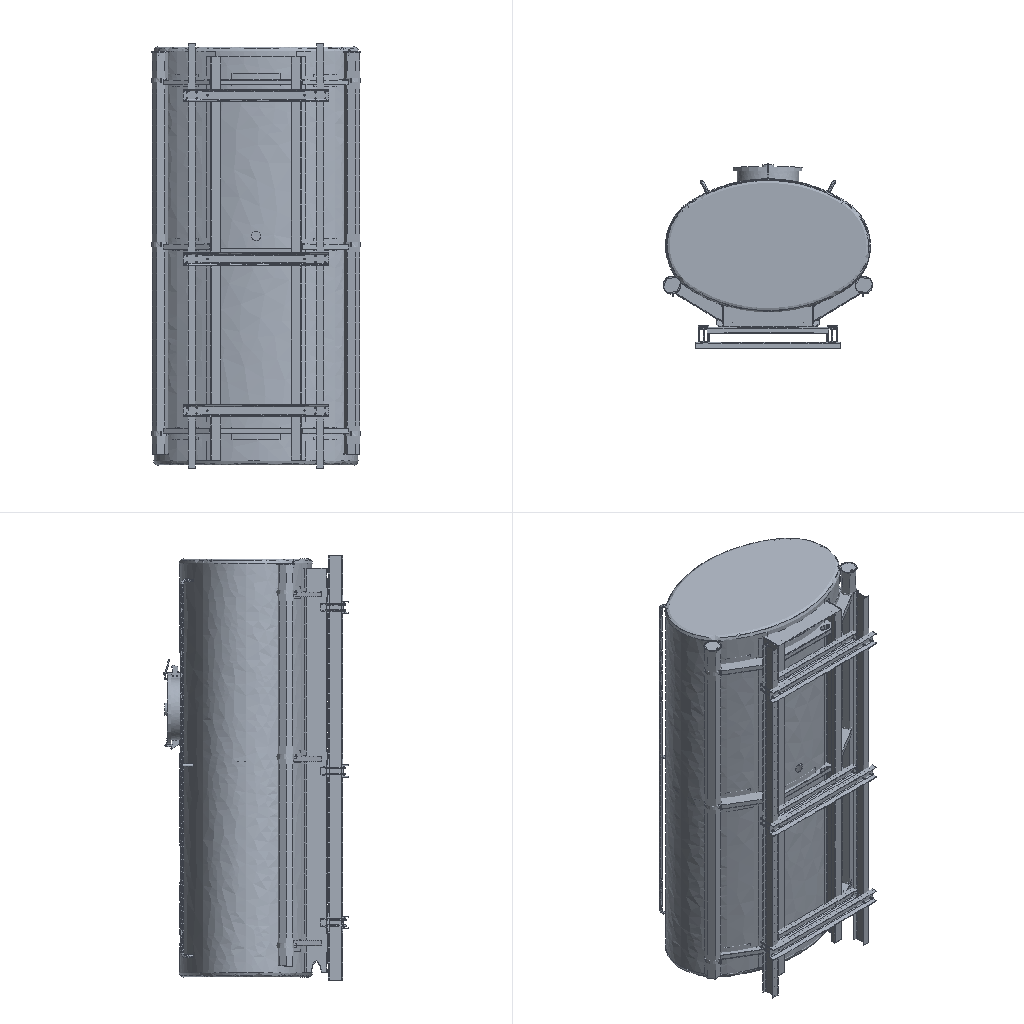Simulation study | ansys workbench
Ansys APDL input file, long lists of numbers shortened:
/batch
/config,noeldb,1     ! force off writing results to database
*get,_wallstrt,active,,time,wall
! ANSYS input file written by Workbench version 2022 R1
! File used for geometry attach: F:\ansys（分析文件汇总)\洒水车有限元分析\晒水车罐体.STEP
/title,wbnew--____ 2 (E5)
! ****** Begin Custom Load Command Snippet ******
/COM, ACT Extensions:
/COM,     LSDYNA, 2021.1
/COM,
! ****** End   Custom Load Command Snippet ******
*DIM,_wb_ProjectScratch_dir,string,248
_wb_ProjectScratch_dir(1) = 'C:\Users\Administrator\AppData\Local\Temp\WB_Administrator_19044_2\_ProjectScratch\Scr5F41\'
*DIM,_wb_SolverFiles_dir,string,248
_wb_SolverFiles_dir(1) = 'C:\Users\Administrator\AppData\Local\Temp\WB_Administrator_19044_2\wbnew_files\dp0\SYS-3\MECH\'
*DIM,_wb_userfiles_dir,string,248
_wb_userfiles_dir(1) = 'C:\Users\Administrator\AppData\Local\Temp\WB_Administrator_19044_2\wbnew_files\user_files\'
/com,--- Data in consistent NMM units. See Solving Units in the help system for more information.
/units,MPA
/nopr
/wb,file,start              !  signify a WB generated input file
/prep7
! Turn off shape checking because checks already performed inside WB mesher.
! See help system for more information.
SHPP,OFF,,NOWARN
/nolist
etcon,set             ! allow ANSYS to choose best KEYOP's for 180x elements, resets any applicable keyopt to MAPDL defaults
/com,*********** Nodes for the whole assembly ***********
nblock,3,,154514
(1i9,3e20.9e3)
    59613    -4.978285790E+02     4.306437121E+02     3.184288870E+01
! (140467 more lines like these left out)
-1
/wb,elem,start            !  set before creation of elements
/com,*********** Elements for Body 1 "__|1210-011-G03|__-__1" ***********
et,1,187
eblock,19,solid,,5134
(19i9)
        1        1        1        1        0        0        0        0       10        0        1     1367     1730     1457     1374     9329     9682     9325     9324
! (10267 more lines like these left out)
-1
/com,*********** Elements for Body 2 "__|1210-011-G03|__-__1[2]" ***********
et,2,187
eblock,19,solid,,5134
(19i9)
        2        2        2        2        0        0        0        0       10        0     5135    12093    12456    12183    12100    20055    20408    20051    20050
! (10267 more lines like these left out)
-1
/com,*********** Elements for Body 3 "__|__-0|__-__3" ***********
et,3,187
eblock,19,solid,,12299
(19i9)
        3        3        3        3        0        0        0        0       10        0    10269    22599    23787    23678    22852    33647    40850    33645    33640
! (24597 more lines like these left out)
-1
/com,*********** Elements for Body 4 "__|1210-041-G03|__-__9" ***********
et,4,187
eblock,19,solid,,1630
(19i9)
        4        4        4        4        0        0        0        0       10        0    22568    46545    47052    46995    46688    47336    49436    47333    47330
! (3259 more lines like these left out)
-1
/com,*********** Elements for Body 5 "__|1210-042-G03|__-__1" ***********
et,5,186
keyo,5,2,1          ! set full integration on SOLID186
eblock,19,solid,,62
(19i9)
        5        5        5        5        0        0        0        0       20        0    24198    50489    50500    50499    50490    50548    50537    50538    50539
! (123 more lines like these left out)
-1
! (74 more sections like these left out)
/wb,elem,end               !  done creating elements
/com,*********** Send User Defined Coordinate System(s) ***********
csys,0
toffst,273.15,  ! Temperature offset from absolute zero
/com,*********** Set Reference Temperature ***********
tref,22.
/wb,mat,start              !  starting to send materials
/com,*********** Send Materials ***********
Temperature = 'TEMP' ! Temperature
MP,DENS,1,7.85e-09,	! tonne mm^-3
MP,ALPX,1,1.2e-05,	! C^-1
MP,C,1,434000000,	! mm^2 s^-2 C^-1
MP,KXX,1,60.5,	! tonne mm s^-3 C^-1
MP,RSVX,1,0.00017,	! ohm mm
MP,EX,1,200000,	! tonne s^-2 mm^-1
MP,NUXY,1,0.3,
MP,MURX,1,10000,
Temperature = 'TEMP' ! Temperature
MP,DENS,2,7.85e-09,	! tonne mm^-3
MP,ALPX,2,1.2e-05,	! C^-1
MP,C,2,434000000,	! mm^2 s^-2 C^-1
MP,KXX,2,60.5,	! tonne mm s^-3 C^-1
MP,RSVX,2,0.00017,	! ohm mm
MP,EX,2,200000,	! tonne s^-2 mm^-1
MP,NUXY,2,0.3,
MP,MURX,2,10000,
Temperature = 'TEMP' ! Temperature
MP,DENS,3,7.85e-09,	! tonne mm^-3
MP,ALPX,3,1.2e-05,	! C^-1
MP,C,3,434000000,	! mm^2 s^-2 C^-1
MP,KXX,3,60.5,	! tonne mm s^-3 C^-1
MP,RSVX,3,0.00017,	! ohm mm
MP,EX,3,200000,	! tonne s^-2 mm^-1
MP,NUXY,3,0.3,
MP,MURX,3,10000,
Temperature = 'TEMP' ! Temperature
MP,DENS,4,7.85e-09,	! tonne mm^-3
MP,ALPX,4,1.2e-05,	! C^-1
MP,C,4,434000000,	! mm^2 s^-2 C^-1
MP,KXX,4,60.5,	! tonne mm s^-3 C^-1
MP,RSVX,4,0.00017,	! ohm mm
MP,EX,4,200000,	! tonne s^-2 mm^-1
MP,NUXY,4,0.3,
MP,MURX,4,10000,
Temperature = 'TEMP' ! Temperature
MP,DENS,5,7.85e-09,	! tonne mm^-3
MP,ALPX,5,1.2e-05,	! C^-1
MP,C,5,434000000,	! mm^2 s^-2 C^-1
MP,KXX,5,60.5,	! tonne mm s^-3 C^-1
MP,RSVX,5,0.00017,	! ohm mm
MP,EX,5,200000,	! tonne s^-2 mm^-1
MP,NUXY,5,0.3,
MP,MURX,5,10000,
Temperature = 'TEMP' ! Temperature
MP,DENS,6,7.85e-09,	! tonne mm^-3
MP,ALPX,6,1.2e-05,	! C^-1
MP,C,6,434000000,	! mm^2 s^-2 C^-1
MP,KXX,6,60.5,	! tonne mm s^-3 C^-1
MP,RSVX,6,0.00017,	! ohm mm
MP,EX,6,200000,	! tonne s^-2 mm^-1
MP,NUXY,6,0.3,
MP,MURX,6,10000,
Temperature = 'TEMP' ! Temperature
MP,DENS,7,7.85e-09,	! tonne mm^-3
MP,ALPX,7,1.2e-05,	! C^-1
MP,C,7,434000000,	! mm^2 s^-2 C^-1
MP,KXX,7,60.5,	! tonne mm s^-3 C^-1
MP,RSVX,7,0.00017,	! ohm mm
MP,EX,7,200000,	! tonne s^-2 mm^-1
MP,NUXY,7,0.3,
MP,MURX,7,10000,
Temperature = 'TEMP' ! Temperature
MP,DENS,8,7.85e-09,	! tonne mm^-3
MP,ALPX,8,1.2e-05,	! C^-1
MP,C,8,434000000,	! mm^2 s^-2 C^-1
MP,KXX,8,60.5,	! tonne mm s^-3 C^-1
MP,RSVX,8,0.00017,	! ohm mm
MP,EX,8,200000,	! tonne s^-2 mm^-1
MP,NUXY,8,0.3,
MP,MURX,8,10000,
Temperature = 'TEMP' ! Temperature
MP,DENS,9,7.85e-09,	! tonne mm^-3
MP,ALPX,9,1.2e-05,	! C^-1
MP,C,9,434000000,	! mm^2 s^-2 C^-1
MP,KXX,9,60.5,	! tonne mm s^-3 C^-1
MP,RSVX,9,0.00017,	! ohm mm
MP,EX,9,200000,	! tonne s^-2 mm^-1
! (632 more lines like these left out)
/wb,mat,end                !  done sending materials
!************************* Model Summary ********************
!__|1210-011-G03|__-__1,	Q235B,	matid,	1
!__|1210-011-G03|__-__1[2],	Q235B,	matid,	2
!__|__-0|__-__3,	Q235B,	matid,	3
! (78 more lines like these left out)
*get,_xmin,node,,mnloc,x
*get,_ymin,node,,mnloc,y
*get,_zmin,node,,mnloc,z
*get,_xmax,node,,mxloc,x
*get,_ymax,node,,mxloc,y
*get,_zmax,node,,mxloc,z
_ASMDIAG=(_xmax-_xmin)*(_xmax-_xmin)+(_ymax-_ymin)*(_ymax-_ymin)+(_zmax-_zmin)*(_zmax-_zmin)
_ASMDIAG=SQRT(_ASMDIAG)
/wb,contact,start          !  starting to send contact
/com,*********** Create Contact "接触区域" ***********
/com,            Real Constant Set For Above Contact Is 81 & 80
*set,tid,81
*set,cid,80
r,tid
r,cid
et,tid,170
et,cid,174
eblock,10,,,316
(15i9)
   106793       81       81       81        0      240      526      550      550     3708     5545      550     3709
! (315 more lines like these left out)
-1
eblock,10,,,316
(15i9)
   107109       80       80       80        0      240      526      550      550     3708     5545      550     3709
! (315 more lines like these left out)
-1
eblock,10,,,119
(15i9)
   107425       80       81       80        0    21474    21805    21997    21997    25860    28558    21997    25861
! (118 more lines like these left out)
-1
eblock,10,,,119
(15i9)
   107544       81       80       81        0    21474    21805    21997    21997    25860    28558    21997    25861
! (118 more lines like these left out)
-1
keyo,cid,8,2               ! auto create asymmetric contact (from Program Controlled setting)
keyo,cid,10,0              ! adjust contact stiffness each NR iteration (from Program Controlled setting)
keyo,cid,12,5              ! bonded always
keyo,cid,18,1              ! small sliding turned on by application
keyo,cid,2,0               ! augmented Lagrange (from Program Controlled setting)
keyo,cid,4,0               ! on Gauss point (from Program Controlled setting)
keyo,cid,9,1               ! ignore initial gaps/penetration
keyo,cid,7,0               ! No Prediction
rmod,tid,3,10.      ! FKN
rmod,tid,5,0.       ! ICONT
rmod,tid,6,0.       ! PINB
rmod,tid,10,0.      ! CNOF
rmod,tid,12,0.      ! FKT
rmod,tid,36,260     ! WB DSID
rmod,cid,3,10.      ! FKN
rmod,cid,5,0.       ! ICONT
rmod,cid,6,0.       ! PINB
rmod,cid,10,0.      ! CNOF
rmod,cid,12,0.      ! FKT
rmod,cid,36,260     ! WB DSID
/com,*********** Create Contact "接触区域 2" ***********
/com,            Real Constant Set For Above Contact Is 83 & 82
*set,tid,83
*set,cid,82
r,tid
r,cid
et,tid,170
et,cid,174
eblock,10,,,10
(15i9)
   107663       83       83       83        0      221      499      516      516     3552     5438      516     3554
! (9 more lines like these left out)
-1
eblock,10,,,10
(15i9)
   107673       82       82       82        0      221      499      516      516     3552     5438      516     3554
! (9 more lines like these left out)
-1
eblock,10,,,2
(15i9)
   107683       82       83       82        0    63922    63923    63749    63747    64830    64280    64275    64276
   107684       82       83       82        0    63923    64008    63748    63749    64835    64279    64277    64280
-1
eblock,10,,,2
(15i9)
   107685       83       82       83        0    63922    63923    63749    63747    64830    64280    64275    64276
   107686       83       82       83        0    63923    64008    63748    63749    64835    64279    64277    64280
-1
keyo,cid,8,2               ! auto create asymmetric contact (from Program Controlled setting)
keyo,cid,10,0              ! adjust contact stiffness each NR iteration (from Program Controlled setting)
keyo,cid,12,5              ! bonded always
keyo,cid,18,1              ! small sliding turned on by application
keyo,cid,2,0               ! augmented Lagrange (from Program Controlled setting)
keyo,cid,4,0               ! on Gauss point (from Program Controlled setting)
keyo,cid,9,1               ! ignore initial gaps/penetration
keyo,cid,7,0               ! No Prediction
rmod,tid,3,10.      ! FKN
rmod,tid,5,0.       ! ICONT
rmod,tid,6,0.       ! PINB
rmod,tid,10,0.      ! CNOF
rmod,tid,12,0.      ! FKT
rmod,tid,36,263     ! WB DSID
rmod,cid,3,10.      ! FKN
rmod,cid,5,0.       ! ICONT
rmod,cid,6,0.       ! PINB
rmod,cid,10,0.      ! CNOF
rmod,cid,12,0.      ! FKT
rmod,cid,36,263     ! WB DSID
/com,*********** Create Contact "接触区域 3" ***********
/com,            Real Constant Set For Above Contact Is 85 & 84
*set,tid,85
*set,cid,84
r,tid
r,cid
et,tid,170
et,cid,174
eblock,10,,,27
(15i9)
   107687       85       85       85        0      221      499      516      516     3552     5438      516     3554
! (26 more lines like these left out)
-1
eblock,10,,,27
(15i9)
   107714       84       84       84        0      221      499      516      516     3552     5438      516     3554
! (26 more lines like these left out)
-1
eblock,10,,,173
(15i9)
   107741       84       85       84        0    65546    65628    65630    65630    65873    66412    65630    65874
! (172 more lines like these left out)
-1
eblock,10,,,173
(15i9)
   107914       85       84       85        0    65546    65628    65630    65630    65873    66412    65630    65874
! (172 more lines like these left out)
-1
keyo,cid,8,2               ! auto create asymmetric contact (from Program Controlled setting)
keyo,cid,10,0              ! adjust contact stiffness each NR iteration (from Program Controlled setting)
keyo,cid,12,5              ! bonded always
keyo,cid,18,1              ! small sliding turned on by application
keyo,cid,2,0               ! augmented Lagrange (from Program Controlled setting)
keyo,cid,4,0               ! on Gauss point (from Program Controlled setting)
keyo,cid,9,1               ! ignore initial gaps/penetration
keyo,cid,7,0               ! No Prediction
rmod,tid,3,10.      ! FKN
rmod,tid,5,0.       ! ICONT
rmod,tid,6,0.       ! PINB
rmod,tid,10,0.      ! CNOF
rmod,tid,12,0.      ! FKT
rmod,tid,36,266     ! WB DSID
rmod,cid,3,10.      ! FKN
rmod,cid,5,0.       ! ICONT
rmod,cid,6,0.       ! PINB
rmod,cid,10,0.      ! CNOF
rmod,cid,12,0.      ! FKT
rmod,cid,36,266     ! WB DSID
/com,*********** Create Contact "接触区域 4" ***********
/com,            Real Constant Set For Above Contact Is 87 & 86
*set,tid,87
*set,cid,86
r,tid
r,cid
et,tid,170
et,cid,174
eblock,10,,,33
(15i9)
   108087       87       87       87        0      303      652      668      668     4185     5810      668     4187
! (32 more lines like these left out)
-1
eblock,10,,,33
(15i9)
   108120       86       86       86        0      303      652      668      668     4185     5810      668     4187
! (32 more lines like these left out)
-1
eblock,10,,,34
(15i9)
   108153       86       87       86        0    68869    68866    68870    68870    69399    69400    68870    69417
! (33 more lines like these left out)
-1
eblock,10,,,34
(15i9)
   108187       87       86       87        0    68869    68866    68870    68870    69399    69400    68870    69417
! (33 more lines like these left out)
-1
keyo,cid,8,2               ! auto create asymmetric contact (from Program Controlled setting)
keyo,cid,10,0              ! adjust contact stiffness each NR iteration (from Program Controlled setting)
keyo,cid,12,5              ! bonded always
keyo,cid,18,1              ! small sliding turned on by application
keyo,cid,2,0               ! augmented Lagrange (from Program Controlled setting)
keyo,cid,4,0               ! on Gauss point (from Program Controlled setting)
keyo,cid,9,1               ! ignore initial gaps/penetration
keyo,cid,7,0               ! No Prediction
rmod,tid,3,10.      ! FKN
rmod,tid,5,0.       ! ICONT
rmod,tid,6,0.       ! PINB
rmod,tid,10,0.      ! CNOF
rmod,tid,12,0.      ! FKT
rmod,tid,36,269     ! WB DSID
rmod,cid,3,10.      ! FKN
rmod,cid,5,0.       ! ICONT
rmod,cid,6,0.       ! PINB
rmod,cid,10,0.      ! CNOF
rmod,cid,12,0.      ! FKT
rmod,cid,36,269     ! WB DSID
/com,*********** Create Contact "接触区域 5" ***********
/com,            Real Constant Set For Above Contact Is 89 & 88
*set,tid,89
*set,cid,88
r,tid
r,cid
et,tid,170
et,cid,174
eblock,10,,,11
(15i9)
   108221       89       89       89        0       42      552      528      528     2210     5551      528     2209
! (10 more lines like these left out)
-1
eblock,10,,,11
(15i9)
   108232       88       88       88        0       42      552      528      528     2210     5551      528     2209
! (10 more lines like these left out)
-1
eblock,10,,,1
(15i9)
   108243       88       89       88        0    84030    84031    84032    84033    84160    84162    84163    84161
-1
eblock,10,,,1
(15i9)
   108244       89       88       89        0    84030    84031    84032    84033    84160    84162    84163    84161
-1
keyo,cid,8,2               ! auto create asymmetric contact (from Program Controlled setting)
keyo,cid,10,0              ! adjust contact stiffness each NR iteration (from Program Controlled setting)
keyo,cid,12,5              ! bonded always
keyo,cid,18,1              ! small sliding turned on by application
keyo,cid,2,0               ! augmented Lagrange (from Program Controlled setting)
keyo,cid,4,0               ! on Gauss point (from Program Controlled setting)
keyo,cid,9,1               ! ignore initial gaps/penetration
keyo,cid,7,0               ! No Prediction
rmod,tid,3,10.      ! FKN
rmod,tid,5,0.       ! ICONT
rmod,tid,6,0.       ! PINB
rmod,tid,10,0.      ! CNOF
rmod,tid,12,0.      ! FKT
rmod,tid,36,272     ! WB DSID
rmod,cid,3,10.      ! FKN
rmod,cid,5,0.       ! ICONT
rmod,cid,6,0.       ! PINB
rmod,cid,10,0.      ! CNOF
rmod,cid,12,0.      ! FKT
rmod,cid,36,272     ! WB DSID
! (211 more sections like these left out)
/wb,contact,end            !  done creating contacts
/golist
/wb,load,start             !  starting to send loads
/com,*********** Fixed Supports ***********
CMBLOCK,_FIXEDSU,NODE,    82027
(8i10)
         5         7         8         9       154       155       156       157
! (10253 more lines like these left out)
cmsel,s,_FIXEDSU
d,all,all
nsel,all
/com,*********** Define Pressure Using Surface Effect Elements "__" ***********
et,512,154
eblock,10,,,3608
(15i9)
   141235      512      512      512        0     1482     1618     1715     1715     9837    10417     1715     9840
! (3607 more lines like these left out)
-1
esel,s,type,,512
keyop,512,7,0                ! Use deformed area for application of load
esel,all
esel,all
/gst,on,on
fini
*get,_numnode,node,0,count
*get,_numelem,elem,0,count
*get, _MAXELEMNUM, elem, 0, NUM, MAX
*get, _MAXNODENUM, node, 0, NUM, MAX
*get, _MAXELEMTYPE, etyp, 0, NUM, MAX
*get, _MAXREALCONST, real, 0, NUM, MAX
/go
/wb,load,end               !  done creating loads
/com,--- Number of total nodes = %_numnode%
/com,--- Number of contact elements = 38050
/com,--- Number of spring elements = 0
/com,--- Number of bearing elements = 0
/com,--- Number of solid elements = 58082
/com,--- Number of condensed parts = 0
/com,--- Number of total elements = %_numelem%
*get,_wallbsol,active,,time,wall
/com,****************************************************************************
/com,*************************    SOLUTION       ********************************
/com,****************************************************************************
/solu
antype,0                   ! static analysis
_thickRatio=  0     ! Ratio of thick parts in the model
eqsl,sparse,,,,,1
cntr,print,1               ! print out contact info and also make no initial contact an error
cntr,out,yes               ! write contact output to file.cmn due to many contact pairs present
dmpoption,emat,no             ! Don't combine emat file for DANSYS
dmpoption,esav,no             ! Don't combine esav file for DANSYS
nldiag,cont,iter           ! print out contact info each equilibrium iteration
rescontrol,,none                 ! Do not keep any restart files
/com,****************************************************
/com,******************* SOLVE FOR LS 1 OF 1 ****************
esel,s,type,,512
nsle
sf,all,pres,0.6
nsel,all
esel,all
esel,all
/nopr
/gopr
nsub,1,1,1
time,1.
outres,erase
outres,all,none
outres,nsol,all,
outres,rsol,all
outres,eangl,all
outres,etmp,all
outres,veng,all
outres,strs,all,
outres,epel,all,
outres,eppl,all,
outres,cont,all,
! *********** WB SOLVE COMMAND ***********
! check interactive state
*get,ANSINTER_,active,,int
*if,ANSINTER_,ne,0,then
/eof
*endif
solve
/com *************** Write FE CONNECTORS *********
CEWRITE,file,ce,,INTE
/com,****************************************************
/com,*************** FINISHED SOLVE FOR LS 1 *************
*get,_wallasol,active,,time,wall
/nopr
*get,_numnode,node,0,count
*get,_numelem,elem,0,count
*get, _MAXELEMNUM, elem, 0, NUM, MAX
*get, _MAXNODENUM, node, 0, NUM, MAX,,,INTERNAL
*get, _MAXELEMTYPE, etyp, 0, NUM, MAX
*get, _MAXREALCONST, real, 0, NUM, MAX
/gopr
/post1
xmlo,ENCODING,ISO-8859-1
xmlo,parm
/xml,parm,xml
fini
/gopr
*get,_walldone,active,,time,wall
_preptime=(_wallbsol-_wallstrt)*3600
_solvtime=(_wallasol-_wallbsol)*3600
_posttime=(_walldone-_wallasol)*3600
_totaltim=(_walldone-_wallstrt)*3600
*get,_dlbratio,active,0,solu,dlbr
*get,_combtime,active,0,solu,comb
*get,_ssmode,active,0,solu,ssmm
*get,_ndofs,active,0,solu,ndof
*get,_sol_end_time,active,0,set,time
*if,_sol_end_time,eq,1.,then
/fclean				!clean distributed files
*endif
/com,--- Total number of nodes = %_numnode%
/com,--- Total number of elements = %_numelem%
/com,--- Element load balance ratio = %_dlbratio%
/com,--- Time to combine distributed files = %_combtime%
/com,--- Sparse memory mode = %_ssmode%
/com,--- Number of DOF = %_ndofs%
/wb,file,end               ! done with WB generated input